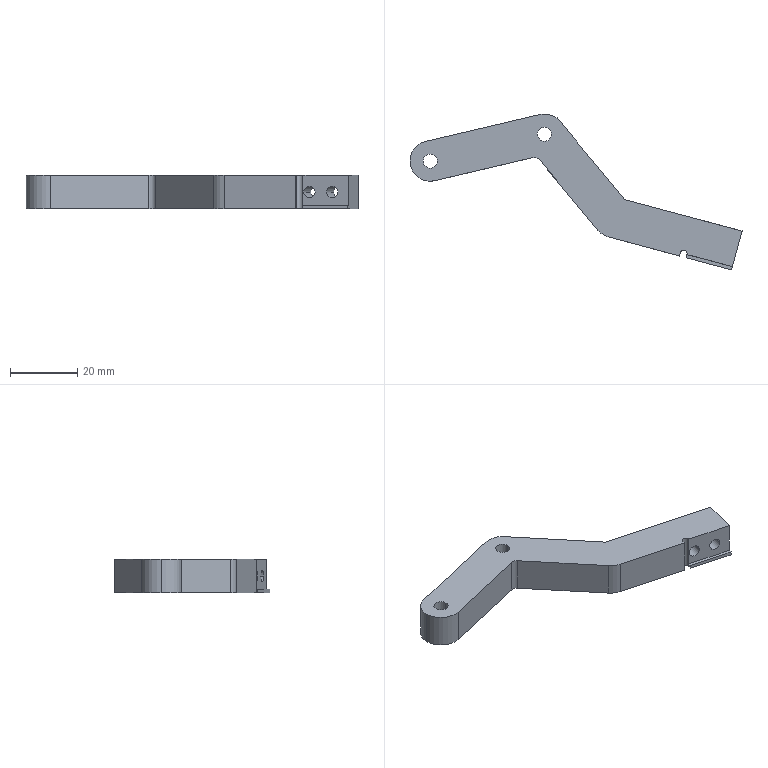Part | STEP file | 02-06 product suction plate b | 1 solid | 39 faces | box 98.778 x 46.377 x 10 mm | volume 12156 mm3 | cylinder 20 | plane 19 | commonest cylinder face diameters 3.5 x4 4.2 x4 12 x4 8 x3 2 x2 10 x2
STEP:
#1=CARTESIAN_POINT('',(35.046,-23.543,5.));
#2=VERTEX_POINT('',#1);
#3=CARTESIAN_POINT('',(38.91,-24.578,9.));
#4=VERTEX_POINT('',#3);
#5=CARTESIAN_POINT('',(38.91,-24.578,5.));
#6=DIRECTION('',(0.2588,0.9659,0.));
#7=DIRECTION('',(-0.9659,0.2588,0.));
#8=AXIS2_PLACEMENT_3D('',#5,#6,#7);
#9=CIRCLE('',#8,4.);
#10=EDGE_CURVE('',#2,#4,#9,.T.);
#11=ORIENTED_EDGE('',*,*,#10,.F.);
#12=CARTESIAN_POINT('',(35.823,-20.645,5.));
#13=VERTEX_POINT('',#12);
#14=CARTESIAN_POINT('',(35.046,-23.543,5.));
#15=DIRECTION('',(0.2588,0.9659,0.));
#16=VECTOR('',#15,1000.);
#17=LINE('',#14,#16);
#18=EDGE_CURVE('',#2,#13,#17,.T.);
#19=ORIENTED_EDGE('',*,*,#18,.T.);
#20=CARTESIAN_POINT('',(39.687,-21.68,9.));
#21=VERTEX_POINT('',#20);
#22=CARTESIAN_POINT('',(39.687,-21.68,5.));
#23=DIRECTION('',(0.2588,0.9659,0.));
#24=DIRECTION('',(-0.9659,0.2588,0.));
#25=AXIS2_PLACEMENT_3D('',#22,#23,#24);
#26=CIRCLE('',#25,4.);
#27=EDGE_CURVE('',#13,#21,#26,.T.);
#28=ORIENTED_EDGE('',*,*,#27,.T.);
#29=CARTESIAN_POINT('',(38.91,-24.578,9.));
#30=DIRECTION('',(0.2588,0.9659,0.));
#31=VECTOR('',#30,1000.);
#32=LINE('',#29,#31);
#33=EDGE_CURVE('',#4,#21,#32,.T.);
#34=ORIENTED_EDGE('',*,*,#33,.F.);
#35=EDGE_LOOP('',(#11,#19,#28,#34));
#36=FACE_OUTER_BOUND('',#35,.T.);
#37=CARTESIAN_POINT('',(38.91,-24.578,5.));
#38=DIRECTION('',(0.2588,0.9659,0.));
#39=DIRECTION('',(-0.9659,0.2588,0.));
#40=AXIS2_PLACEMENT_3D('',#37,#38,#39);
#41=CYLINDRICAL_SURFACE('',#40,4.);
#42=ADVANCED_FACE('',(#36),#41,.F.);
#43=CARTESIAN_POINT('',(34.942,-31.529,0.));
#44=VERTEX_POINT('',#43);
#45=CARTESIAN_POINT('',(32.976,-31.27,0.));
#46=VERTEX_POINT('',#45);
#47=CARTESIAN_POINT('',(33.942,-31.529,0.));
#48=DIRECTION('',(0.,0.,1.));
#49=DIRECTION('',(1.,0.,0.));
#50=AXIS2_PLACEMENT_3D('',#47,#48,#49);
#51=CIRCLE('',#50,1.);
#52=EDGE_CURVE('',#44,#46,#51,.T.);
#53=ORIENTED_EDGE('',*,*,#52,.F.);
#54=CARTESIAN_POINT('',(34.942,-31.529,10.));
#55=VERTEX_POINT('',#54);
#56=CARTESIAN_POINT('',(34.942,-31.529,0.));
#57=DIRECTION('',(0.,0.,1.));
#58=VECTOR('',#57,1000.);
#59=LINE('',#56,#58);
#60=EDGE_CURVE('',#44,#55,#59,.T.);
#61=ORIENTED_EDGE('',*,*,#60,.T.);
#62=CARTESIAN_POINT('',(32.976,-31.27,10.));
#63=VERTEX_POINT('',#62);
#64=CARTESIAN_POINT('',(33.942,-31.529,10.));
#65=DIRECTION('',(0.,0.,1.));
#66=DIRECTION('',(1.,0.,0.));
#67=AXIS2_PLACEMENT_3D('',#64,#65,#66);
#68=CIRCLE('',#67,1.);
#69=EDGE_CURVE('',#55,#63,#68,.T.);
#70=ORIENTED_EDGE('',*,*,#69,.T.);
#71=CARTESIAN_POINT('',(32.976,-31.27,1.));
#72=DIRECTION('',(0.,0.,1.));
#73=VECTOR('',#72,1000.);
#74=LINE('',#71,#73);
#75=EDGE_CURVE('',#46,#63,#74,.T.);
#76=ORIENTED_EDGE('',*,*,#75,.F.);
#77=EDGE_LOOP('',(#53,#61,#70,#76));
#78=FACE_OUTER_BOUND('',#77,.T.);
#79=CARTESIAN_POINT('',(33.942,-31.529,0.));
#80=DIRECTION('',(0.,0.,1.));
#81=DIRECTION('',(1.,0.,0.));
#82=AXIS2_PLACEMENT_3D('',#79,#80,#81);
#83=CYLINDRICAL_SURFACE('',#82,1.);
#84=ADVANCED_FACE('',(#78),#83,.F.);
#85=CARTESIAN_POINT('',(-5.4,4.,10.));
#86=VERTEX_POINT('',#85);
#87=CARTESIAN_POINT('',(-9.6,4.,10.));
#88=VERTEX_POINT('',#87);
#89=CARTESIAN_POINT('',(-7.5,4.,10.));
#90=DIRECTION('',(0.,0.,-1.));
#91=DIRECTION('',(-1.,0.,0.));
#92=AXIS2_PLACEMENT_3D('',#89,#90,#91);
#93=CIRCLE('',#92,2.1);
#94=EDGE_CURVE('',#86,#88,#93,.T.);
#95=ORIENTED_EDGE('',*,*,#94,.F.);
#96=CARTESIAN_POINT('',(-5.4,4.,0.));
#97=VERTEX_POINT('',#96);
#98=CARTESIAN_POINT('',(-5.4,4.,0.));
#99=DIRECTION('',(0.,0.,-1.));
#100=VECTOR('',#99,1000.);
#101=LINE('',#98,#100);
#102=EDGE_CURVE('',#86,#97,#101,.T.);
#103=ORIENTED_EDGE('',*,*,#102,.T.);
#104=CARTESIAN_POINT('',(-9.6,4.,0.));
#105=VERTEX_POINT('',#104);
#106=CARTESIAN_POINT('',(-7.5,4.,0.));
#107=DIRECTION('',(0.,0.,-1.));
#108=DIRECTION('',(-1.,0.,0.));
#109=AXIS2_PLACEMENT_3D('',#106,#107,#108);
#110=CIRCLE('',#109,2.1);
#111=EDGE_CURVE('',#97,#105,#110,.T.);
#112=ORIENTED_EDGE('',*,*,#111,.T.);
#113=CARTESIAN_POINT('',(-9.6,4.,0.));
#114=DIRECTION('',(0.,0.,-1.));
#115=VECTOR('',#114,1000.);
#116=LINE('',#113,#115);
#117=EDGE_CURVE('',#88,#105,#116,.T.);
#118=ORIENTED_EDGE('',*,*,#117,.F.);
#119=EDGE_LOOP('',(#95,#103,#112,#118));
#120=FACE_OUTER_BOUND('',#119,.T.);
#121=CARTESIAN_POINT('',(-7.5,4.,0.));
#122=DIRECTION('',(0.,0.,-1.));
#123=DIRECTION('',(-1.,0.,0.));
#124=AXIS2_PLACEMENT_3D('',#121,#122,#123);
#125=CYLINDRICAL_SURFACE('',#124,2.1);
#126=ADVANCED_FACE('',(#120),#125,.F.);
#127=CARTESIAN_POINT('',(-39.4,-4.,10.));
#128=VERTEX_POINT('',#127);
#129=CARTESIAN_POINT('',(-43.6,-4.,10.));
#130=VERTEX_POINT('',#129);
#131=CARTESIAN_POINT('',(-41.5,-4.,10.));
#132=DIRECTION('',(0.,0.,-1.));
#133=DIRECTION('',(-1.,0.,0.));
#134=AXIS2_PLACEMENT_3D('',#131,#132,#133);
#135=CIRCLE('',#134,2.1);
#136=EDGE_CURVE('',#128,#130,#135,.T.);
#137=ORIENTED_EDGE('',*,*,#136,.F.);
#138=CARTESIAN_POINT('',(-39.4,-4.,1.3));
#139=VERTEX_POINT('',#138);
#140=CARTESIAN_POINT('',(-39.4,-4.,0.));
#141=DIRECTION('',(0.,0.,-1.));
#142=VECTOR('',#141,1000.);
#143=LINE('',#140,#142);
#144=EDGE_CURVE('',#128,#139,#143,.T.);
#145=ORIENTED_EDGE('',*,*,#144,.T.);
#146=CARTESIAN_POINT('',(-43.6,-4.,1.3));
#147=VERTEX_POINT('',#146);
#148=CARTESIAN_POINT('',(-41.5,-4.,1.3));
#149=DIRECTION('',(0.,0.,-1.));
#150=DIRECTION('',(-1.,0.,0.));
#151=AXIS2_PLACEMENT_3D('',#148,#149,#150);
#152=CIRCLE('',#151,2.1);
#153=EDGE_CURVE('',#139,#147,#152,.T.);
#154=ORIENTED_EDGE('',*,*,#153,.T.);
#155=CARTESIAN_POINT('',(-43.6,-4.,0.));
#156=DIRECTION('',(0.,0.,-1.));
#157=VECTOR('',#156,1000.);
#158=LINE('',#155,#157);
#159=EDGE_CURVE('',#130,#147,#158,.T.);
#160=ORIENTED_EDGE('',*,*,#159,.F.);
#161=EDGE_LOOP('',(#137,#145,#154,#160));
#162=FACE_OUTER_BOUND('',#161,.T.);
#163=CARTESIAN_POINT('',(-41.5,-4.,0.));
#164=DIRECTION('',(0.,0.,-1.));
#165=DIRECTION('',(-1.,0.,0.));
#166=AXIS2_PLACEMENT_3D('',#163,#164,#165);
#167=CYLINDRICAL_SURFACE('',#166,2.1);
#168=ADVANCED_FACE('',(#162),#167,.F.);
#169=CARTESIAN_POINT('',(-36.5,-4.,1.3));
#170=VERTEX_POINT('',#169);
#171=CARTESIAN_POINT('',(-46.5,-4.,1.3));
#172=VERTEX_POINT('',#171);
#173=CARTESIAN_POINT('',(-41.5,-4.,1.3));
#174=DIRECTION('',(0.,0.,-1.));
#175=DIRECTION('',(-1.,0.,0.));
#176=AXIS2_PLACEMENT_3D('',#173,#174,#175);
#177=CIRCLE('',#176,5.);
#178=EDGE_CURVE('',#170,#172,#177,.T.);
#179=ORIENTED_EDGE('',*,*,#178,.F.);
#180=CARTESIAN_POINT('',(-36.5,-4.,0.));
#181=VERTEX_POINT('',#180);
#182=CARTESIAN_POINT('',(-36.5,-4.,1.3));
#183=DIRECTION('',(0.,0.,-1.));
#184=VECTOR('',#183,1000.);
#185=LINE('',#182,#184);
#186=EDGE_CURVE('',#170,#181,#185,.T.);
#187=ORIENTED_EDGE('',*,*,#186,.T.);
#188=CARTESIAN_POINT('',(-46.5,-4.,0.));
#189=VERTEX_POINT('',#188);
#190=CARTESIAN_POINT('',(-41.5,-4.,0.));
#191=DIRECTION('',(0.,0.,-1.));
#192=DIRECTION('',(-1.,0.,0.));
#193=AXIS2_PLACEMENT_3D('',#190,#191,#192);
#194=CIRCLE('',#193,5.);
#195=EDGE_CURVE('',#181,#189,#194,.T.);
#196=ORIENTED_EDGE('',*,*,#195,.T.);
#197=CARTESIAN_POINT('',(-46.5,-4.,1.3));
#198=DIRECTION('',(0.,0.,-1.));
#199=VECTOR('',#198,1000.);
#200=LINE('',#197,#199);
#201=EDGE_CURVE('',#172,#189,#200,.T.);
#202=ORIENTED_EDGE('',*,*,#201,.F.);
#203=EDGE_LOOP('',(#179,#187,#196,#202));
#204=FACE_OUTER_BOUND('',#203,.T.);
#205=CARTESIAN_POINT('',(-41.5,-4.,1.3));
#206=DIRECTION('',(0.,0.,-1.));
#207=DIRECTION('',(-1.,0.,0.));
#208=AXIS2_PLACEMENT_3D('',#205,#206,#207);
#209=CYLINDRICAL_SURFACE('',#208,5.);
#210=ADVANCED_FACE('',(#204),#209,.F.);
#211=CARTESIAN_POINT('',(-40.126,-9.841,10.));
#212=VERTEX_POINT('',#211);
#213=CARTESIAN_POINT('',(-47.5,-4.,10.));
#214=VERTEX_POINT('',#213);
#215=CARTESIAN_POINT('',(-41.5,-4.,10.));
#216=DIRECTION('',(0.,0.,-1.));
#217=DIRECTION('',(-1.,0.,0.));
#218=AXIS2_PLACEMENT_3D('',#215,#216,#217);
#219=CIRCLE('',#218,6.);
#220=EDGE_CURVE('',#212,#214,#219,.T.);
#221=ORIENTED_EDGE('',*,*,#220,.T.);
#222=CARTESIAN_POINT('',(-47.5,-4.,0.));
#223=VERTEX_POINT('',#222);
#224=CARTESIAN_POINT('',(-47.5,-4.,10.));
#225=DIRECTION('',(0.,0.,-1.));
#226=VECTOR('',#225,1000.);
#227=LINE('',#224,#226);
#228=EDGE_CURVE('',#214,#223,#227,.T.);
#229=ORIENTED_EDGE('',*,*,#228,.T.);
#230=CARTESIAN_POINT('',(-40.126,-9.841,0.));
#231=VERTEX_POINT('',#230);
#232=CARTESIAN_POINT('',(-41.5,-4.,0.));
#233=DIRECTION('',(0.,0.,-1.));
#234=DIRECTION('',(-1.,0.,0.));
#235=AXIS2_PLACEMENT_3D('',#232,#233,#234);
#236=CIRCLE('',#235,6.);
#237=EDGE_CURVE('',#231,#223,#236,.T.);
#238=ORIENTED_EDGE('',*,*,#237,.F.);
#239=CARTESIAN_POINT('',(-40.126,-9.841,10.));
#240=DIRECTION('',(0.,0.,-1.));
#241=VECTOR('',#240,1000.);
#242=LINE('',#239,#241);
#243=EDGE_CURVE('',#212,#231,#242,.T.);
#244=ORIENTED_EDGE('',*,*,#243,.F.);
#245=EDGE_LOOP('',(#221,#229,#238,#244));
#246=FACE_OUTER_BOUND('',#245,.T.);
#247=CARTESIAN_POINT('',(-41.5,-4.,10.));
#248=DIRECTION('',(0.,0.,-1.));
#249=DIRECTION('',(-1.,0.,0.));
#250=AXIS2_PLACEMENT_3D('',#247,#248,#249);
#251=CYLINDRICAL_SURFACE('',#250,6.);
#252=ADVANCED_FACE('',(#246),#251,.T.);
#253=CARTESIAN_POINT('',(45.291,-34.57,5.));
#254=VERTEX_POINT('',#253);
#255=CARTESIAN_POINT('',(41.911,-33.664,5.));
#256=VERTEX_POINT('',#255);
#257=CARTESIAN_POINT('',(43.601,-34.117,5.));
#258=DIRECTION('',(0.2588,0.9659,0.));
#259=DIRECTION('',(-0.9659,0.2588,0.));
#260=AXIS2_PLACEMENT_3D('',#257,#258,#259);
#261=CIRCLE('',#260,1.75);
#262=EDGE_CURVE('',#254,#256,#261,.T.);
#263=ORIENTED_EDGE('',*,*,#262,.F.);
#264=CARTESIAN_POINT('',(47.362,-26.842,5.));
#265=VERTEX_POINT('',#264);
#266=CARTESIAN_POINT('',(44.256,-38.434,5.));
#267=DIRECTION('',(0.2588,0.9659,0.));
#268=VECTOR('',#267,1000.);
#269=LINE('',#266,#268);
#270=EDGE_CURVE('',#254,#265,#269,.T.);
#271=ORIENTED_EDGE('',*,*,#270,.T.);
#272=CARTESIAN_POINT('',(43.981,-25.937,5.));
#273=VERTEX_POINT('',#272);
#274=CARTESIAN_POINT('',(45.672,-26.39,5.));
#275=DIRECTION('',(-0.2588,-0.9659,0.));
#276=DIRECTION('',(-0.9659,0.2588,0.));
#277=AXIS2_PLACEMENT_3D('',#274,#275,#276);
#278=CIRCLE('',#277,1.75);
#279=EDGE_CURVE('',#273,#265,#278,.T.);
#280=ORIENTED_EDGE('',*,*,#279,.F.);
#281=CARTESIAN_POINT('',(40.875,-37.528,5.));
#282=DIRECTION('',(0.2588,0.9659,0.));
#283=VECTOR('',#282,1000.);
#284=LINE('',#281,#283);
#285=EDGE_CURVE('',#256,#273,#284,.T.);
#286=ORIENTED_EDGE('',*,*,#285,.F.);
#287=EDGE_LOOP('',(#263,#271,#280,#286));
#288=FACE_OUTER_BOUND('',#287,.T.);
#289=CARTESIAN_POINT('',(42.566,-37.981,5.));
#290=DIRECTION('',(0.2588,0.9659,0.));
#291=DIRECTION('',(-0.9659,0.2588,0.));
#292=AXIS2_PLACEMENT_3D('',#289,#290,#291);
#293=CYLINDRICAL_SURFACE('',#292,1.75);
#294=ADVANCED_FACE('',(#288),#293,.F.);
#295=CARTESIAN_POINT('',(38.53,-32.758,5.));
#296=VERTEX_POINT('',#295);
#297=CARTESIAN_POINT('',(35.149,-31.852,5.));
#298=VERTEX_POINT('',#297);
#299=CARTESIAN_POINT('',(36.84,-32.305,5.));
#300=DIRECTION('',(0.2588,0.9659,0.));
#301=DIRECTION('',(-0.9659,0.2588,0.));
#302=AXIS2_PLACEMENT_3D('',#299,#300,#301);
#303=CIRCLE('',#302,1.75);
#304=EDGE_CURVE('',#296,#298,#303,.T.);
#305=ORIENTED_EDGE('',*,*,#304,.F.);
#306=CARTESIAN_POINT('',(40.601,-25.031,5.));
#307=VERTEX_POINT('',#306);
#308=CARTESIAN_POINT('',(37.495,-36.622,5.));
#309=DIRECTION('',(0.2588,0.9659,0.));
#310=VECTOR('',#309,1000.);
#311=LINE('',#308,#310);
#312=EDGE_CURVE('',#296,#307,#311,.T.);
#313=ORIENTED_EDGE('',*,*,#312,.T.);
#314=CARTESIAN_POINT('',(37.22,-24.125,5.));
#315=VERTEX_POINT('',#314);
#316=CARTESIAN_POINT('',(38.91,-24.578,5.));
#317=DIRECTION('',(-0.2588,-0.9659,0.));
#318=DIRECTION('',(-0.9659,0.2588,0.));
#319=AXIS2_PLACEMENT_3D('',#316,#317,#318);
#320=CIRCLE('',#319,1.75);
#321=EDGE_CURVE('',#315,#307,#320,.T.);
#322=ORIENTED_EDGE('',*,*,#321,.F.);
#323=CARTESIAN_POINT('',(34.114,-35.716,5.));
#324=DIRECTION('',(0.2588,0.9659,0.));
#325=VECTOR('',#324,1000.);
#326=LINE('',#323,#325);
#327=EDGE_CURVE('',#298,#315,#326,.T.);
#328=ORIENTED_EDGE('',*,*,#327,.F.);
#329=EDGE_LOOP('',(#305,#313,#322,#328));
#330=FACE_OUTER_BOUND('',#329,.T.);
#331=CARTESIAN_POINT('',(35.804,-36.169,5.));
#332=DIRECTION('',(0.2588,0.9659,0.));
#333=DIRECTION('',(-0.9659,0.2588,0.));
#334=AXIS2_PLACEMENT_3D('',#331,#332,#333);
#335=CYLINDRICAL_SURFACE('',#334,1.75);
#336=ADVANCED_FACE('',(#330),#335,.F.);
#337=ORIENTED_EDGE('',*,*,#312,.F.);
#338=CARTESIAN_POINT('',(36.84,-32.305,5.));
#339=DIRECTION('',(0.2588,0.9659,0.));
#340=DIRECTION('',(-0.9659,0.2588,0.));
#341=AXIS2_PLACEMENT_3D('',#338,#339,#340);
#342=CIRCLE('',#341,1.75);
#343=EDGE_CURVE('',#298,#296,#342,.T.);
#344=ORIENTED_EDGE('',*,*,#343,.F.);
#345=ORIENTED_EDGE('',*,*,#327,.T.);
#346=CARTESIAN_POINT('',(38.91,-24.578,5.));
#347=DIRECTION('',(-0.2588,-0.9659,0.));
#348=DIRECTION('',(-0.9659,0.2588,0.));
#349=AXIS2_PLACEMENT_3D('',#346,#347,#348);
#350=CIRCLE('',#349,1.75);
#351=EDGE_CURVE('',#307,#315,#350,.T.);
#352=ORIENTED_EDGE('',*,*,#351,.F.);
#353=EDGE_LOOP('',(#337,#344,#345,#352));
#354=FACE_OUTER_BOUND('',#353,.T.);
#355=CARTESIAN_POINT('',(35.804,-36.169,5.));
#356=DIRECTION('',(0.2588,0.9659,0.));
#357=DIRECTION('',(-0.9659,0.2588,0.));
#358=AXIS2_PLACEMENT_3D('',#355,#356,#357);
#359=CYLINDRICAL_SURFACE('',#358,1.75);
#360=ADVANCED_FACE('',(#354),#359,.F.);
#361=ORIENTED_EDGE('',*,*,#270,.F.);
#362=CARTESIAN_POINT('',(43.601,-34.117,5.));
#363=DIRECTION('',(0.2588,0.9659,0.));
#364=DIRECTION('',(-0.9659,0.2588,0.));
#365=AXIS2_PLACEMENT_3D('',#362,#363,#364);
#366=CIRCLE('',#365,1.75);
#367=EDGE_CURVE('',#256,#254,#366,.T.);
#368=ORIENTED_EDGE('',*,*,#367,.F.);
#369=ORIENTED_EDGE('',*,*,#285,.T.);
#370=CARTESIAN_POINT('',(45.672,-26.39,5.));
#371=DIRECTION('',(-0.2588,-0.9659,0.));
#372=DIRECTION('',(-0.9659,0.2588,0.));
#373=AXIS2_PLACEMENT_3D('',#370,#371,#372);
#374=CIRCLE('',#373,1.75);
#375=EDGE_CURVE('',#265,#273,#374,.T.);
#376=ORIENTED_EDGE('',*,*,#375,.F.);
#377=EDGE_LOOP('',(#361,#368,#369,#376));
#378=FACE_OUTER_BOUND('',#377,.T.);
#379=CARTESIAN_POINT('',(42.566,-37.981,5.));
#380=DIRECTION('',(0.2588,0.9659,0.));
#381=DIRECTION('',(-0.9659,0.2588,0.));
#382=AXIS2_PLACEMENT_3D('',#379,#380,#381);
#383=CYLINDRICAL_SURFACE('',#382,1.75);
#384=ADVANCED_FACE('',(#378),#383,.F.);
#385=CARTESIAN_POINT('',(34.649,-32.754,0.));
#386=VERTEX_POINT('',#385);
#387=CARTESIAN_POINT('',(34.649,-32.754,1.));
#388=VERTEX_POINT('',#387);
#389=CARTESIAN_POINT('',(34.649,-32.754,10.));
#390=DIRECTION('',(0.,0.,1.));
#391=VECTOR('',#390,1000.);
#392=LINE('',#389,#391);
#393=EDGE_CURVE('',#386,#388,#392,.T.);
#394=ORIENTED_EDGE('',*,*,#393,.F.);
#395=CARTESIAN_POINT('',(48.172,-36.377,0.));
#396=VERTEX_POINT('',#395);
#397=CARTESIAN_POINT('',(48.172,-36.377,0.));
#398=DIRECTION('',(-0.9659,0.2588,0.));
#399=VECTOR('',#398,1000.);
#400=LINE('',#397,#399);
#401=EDGE_CURVE('',#396,#386,#400,.T.);
#402=ORIENTED_EDGE('',*,*,#401,.F.);
#403=CARTESIAN_POINT('',(48.172,-36.377,1.));
#404=VERTEX_POINT('',#403);
#405=CARTESIAN_POINT('',(48.172,-36.377,10.));
#406=DIRECTION('',(0.,0.,-1.));
#407=VECTOR('',#406,1000.);
#408=LINE('',#405,#407);
#409=EDGE_CURVE('',#404,#396,#408,.T.);
#410=ORIENTED_EDGE('',*,*,#409,.F.);
#411=CARTESIAN_POINT('',(32.717,-32.236,1.));
#412=DIRECTION('',(0.9659,-0.2588,0.));
#413=VECTOR('',#412,1000.);
#414=LINE('',#411,#413);
#415=EDGE_CURVE('',#388,#404,#414,.T.);
#416=ORIENTED_EDGE('',*,*,#415,.F.);
#417=EDGE_LOOP('',(#394,#402,#410,#416));
#418=FACE_OUTER_BOUND('',#417,.T.);
#419=CARTESIAN_POINT('',(48.172,-36.377,10.));
#420=DIRECTION('',(-0.2588,-0.9659,0.));
#421=DIRECTION('',(0.9659,-0.2588,0.));
#422=AXIS2_PLACEMENT_3D('',#419,#420,#421);
#423=PLANE('',#422);
#424=ADVANCED_FACE('',(#418),#423,.T.);
#425=CARTESIAN_POINT('',(32.717,-32.236,0.));
#426=VERTEX_POINT('',#425);
#427=CARTESIAN_POINT('',(11.467,-26.542,0.));
#428=VERTEX_POINT('',#427);
#429=CARTESIAN_POINT('',(48.172,-36.377,0.));
#430=DIRECTION('',(-0.9659,0.2588,0.));
#431=VECTOR('',#430,1000.);
#432=LINE('',#429,#431);
#433=EDGE_CURVE('',#426,#428,#432,.T.);
#434=ORIENTED_EDGE('',*,*,#433,.F.);
#435=CARTESIAN_POINT('',(32.717,-32.236,10.));
#436=VERTEX_POINT('',#435);
#437=CARTESIAN_POINT('',(32.717,-32.236,1.));
#438=DIRECTION('',(0.,0.,1.));
#439=VECTOR('',#438,1000.);
#440=LINE('',#437,#439);
#441=EDGE_CURVE('',#426,#436,#440,.T.);
#442=ORIENTED_EDGE('',*,*,#441,.T.);
#443=CARTESIAN_POINT('',(11.467,-26.542,10.));
#444=VERTEX_POINT('',#443);
#445=CARTESIAN_POINT('',(48.172,-36.377,10.));
#446=DIRECTION('',(-0.9659,0.2588,0.));
#447=VECTOR('',#446,1000.);
#448=LINE('',#445,#447);
#449=EDGE_CURVE('',#436,#444,#448,.T.);
#450=ORIENTED_EDGE('',*,*,#449,.T.);
#451=CARTESIAN_POINT('',(11.467,-26.542,10.));
#452=DIRECTION('',(0.,0.,-1.));
#453=VECTOR('',#452,1000.);
#454=LINE('',#451,#453);
#455=EDGE_CURVE('',#444,#428,#454,.T.);
#456=ORIENTED_EDGE('',*,*,#455,.T.);
#457=EDGE_LOOP('',(#434,#442,#450,#456));
#458=FACE_OUTER_BOUND('',#457,.T.);
#459=CARTESIAN_POINT('',(48.172,-36.377,10.));
#460=DIRECTION('',(-0.2588,-0.9659,0.));
#461=DIRECTION('',(0.9659,-0.2588,0.));
#462=AXIS2_PLACEMENT_3D('',#459,#460,#461);
#463=PLANE('',#462);
#464=ADVANCED_FACE('',(#458),#463,.T.);
#465=CARTESIAN_POINT('',(48.431,-35.411,1.));
#466=VERTEX_POINT('',#465);
#467=CARTESIAN_POINT('',(48.431,-35.411,10.));
#468=VERTEX_POINT('',#467);
#469=CARTESIAN_POINT('',(48.431,-35.411,1.));
#470=DIRECTION('',(0.,0.,1.));
#471=VECTOR('',#470,1000.);
#472=LINE('',#469,#471);
#473=EDGE_CURVE('',#466,#468,#472,.T.);
#474=ORIENTED_EDGE('',*,*,#473,.F.);
#475=CARTESIAN_POINT('',(48.172,-36.377,1.));
#476=DIRECTION('',(0.2588,0.9659,0.));
#477=VECTOR('',#476,1000.);
#478=LINE('',#475,#477);
#479=EDGE_CURVE('',#404,#466,#478,.T.);
#480=ORIENTED_EDGE('',*,*,#479,.F.);
#481=ORIENTED_EDGE('',*,*,#409,.T.);
#482=CARTESIAN_POINT('',(51.278,-24.786,0.));
#483=VERTEX_POINT('',#482);
#484=CARTESIAN_POINT('',(53.31,-17.202,0.));
#485=DIRECTION('',(-0.2588,-0.9659,0.));
#486=VECTOR('',#485,1000.);
#487=LINE('',#484,#486);
#488=EDGE_CURVE('',#483,#396,#487,.T.);
#489=ORIENTED_EDGE('',*,*,#488,.F.);
#490=CARTESIAN_POINT('',(51.278,-24.786,10.));
#491=VERTEX_POINT('',#490);
#492=CARTESIAN_POINT('',(51.278,-24.786,0.));
#493=DIRECTION('',(0.,0.,1.));
#494=VECTOR('',#493,1000.);
#495=LINE('',#492,#494);
#496=EDGE_CURVE('',#483,#491,#495,.T.);
#497=ORIENTED_EDGE('',*,*,#496,.T.);
#498=CARTESIAN_POINT('',(53.31,-17.202,10.));
#499=DIRECTION('',(-0.2588,-0.9659,0.));
#500=VECTOR('',#499,1000.);
#501=LINE('',#498,#500);
#502=EDGE_CURVE('',#491,#468,#501,.T.);
#503=ORIENTED_EDGE('',*,*,#502,.T.);
#504=EDGE_LOOP('',(#474,#480,#481,#489,#497,#503));
#505=FACE_OUTER_BOUND('',#504,.T.);
#506=CARTESIAN_POINT('',(53.31,-17.202,10.));
#507=DIRECTION('',(0.9659,-0.2588,0.));
#508=DIRECTION('',(0.2588,0.9659,0.));
#509=AXIS2_PLACEMENT_3D('',#506,#507,#508);
#510=PLANE('',#509);
#511=ADVANCED_FACE('',(#505),#510,.T.);
#512=CARTESIAN_POINT('',(-5.005,9.457,0.));
#513=VERTEX_POINT('',#512);
#514=CARTESIAN_POINT('',(-3.757,8.886,0.));
#515=VERTEX_POINT('',#514);
#516=CARTESIAN_POINT('',(-6.874,10.311,0.));
#517=DIRECTION('',(0.9095,-0.4158,0.));
#518=VECTOR('',#517,1000.);
#519=LINE('',#516,#518);
#520=EDGE_CURVE('',#513,#515,#519,.T.);
#521=ORIENTED_EDGE('',*,*,#520,.F.);
#522=CARTESIAN_POINT('',(-5.005,9.457,10.));
#523=VERTEX_POINT('',#522);
#524=CARTESIAN_POINT('',(-5.005,9.457,10.));
#525=DIRECTION('',(0.,0.,1.));
#526=VECTOR('',#525,1000.);
#527=LINE('',#524,#526);
#528=EDGE_CURVE('',#513,#523,#527,.T.);
#529=ORIENTED_EDGE('',*,*,#528,.T.);
#530=CARTESIAN_POINT('',(-3.757,8.886,10.));
#531=VERTEX_POINT('',#530);
#532=CARTESIAN_POINT('',(-6.874,10.311,10.));
#533=DIRECTION('',(0.9095,-0.4158,0.));
#534=VECTOR('',#533,1000.);
#535=LINE('',#532,#534);
#536=EDGE_CURVE('',#523,#531,#535,.T.);
#537=ORIENTED_EDGE('',*,*,#536,.T.);
#538=CARTESIAN_POINT('',(-3.757,8.886,0.));
#539=DIRECTION('',(0.,0.,1.));
#540=VECTOR('',#539,1000.);
#541=LINE('',#538,#540);
#542=EDGE_CURVE('',#515,#531,#541,.T.);
#543=ORIENTED_EDGE('',*,*,#542,.F.);
#544=EDGE_LOOP('',(#521,#529,#537,#543));
#545=FACE_OUTER_BOUND('',#544,.T.);
#546=CARTESIAN_POINT('',(-6.874,10.311,10.));
#547=DIRECTION('',(0.4158,0.9095,0.));
#548=DIRECTION('',(-0.9095,0.4158,0.));
#549=AXIS2_PLACEMENT_3D('',#546,#547,#548);
#550=PLANE('',#549);
#551=ADVANCED_FACE('',(#545),#550,.T.);
#552=CARTESIAN_POINT('',(-42.874,1.841,10.));
#553=VERTEX_POINT('',#552);
#554=CARTESIAN_POINT('',(-8.874,9.841,10.));
#555=VERTEX_POINT('',#554);
#556=CARTESIAN_POINT('',(-42.874,1.841,10.));
#557=DIRECTION('',(0.9734,0.229,0.));
#558=VECTOR('',#557,1000.);
#559=LINE('',#556,#558);
#560=EDGE_CURVE('',#553,#555,#559,.T.);
#561=ORIENTED_EDGE('',*,*,#560,.T.);
#562=CARTESIAN_POINT('',(-8.874,9.841,0.));
#563=VERTEX_POINT('',#562);
#564=CARTESIAN_POINT('',(-8.874,9.841,10.));
#565=DIRECTION('',(0.,0.,-1.));
#566=VECTOR('',#565,1000.);
#567=LINE('',#564,#566);
#568=EDGE_CURVE('',#555,#563,#567,.T.);
#569=ORIENTED_EDGE('',*,*,#568,.T.);
#570=CARTESIAN_POINT('',(-42.874,1.841,0.));
#571=VERTEX_POINT('',#570);
#572=CARTESIAN_POINT('',(-42.874,1.841,0.));
#573=DIRECTION('',(0.9734,0.229,0.));
#574=VECTOR('',#573,1000.);
#575=LINE('',#572,#574);
#576=EDGE_CURVE('',#571,#563,#575,.T.);
#577=ORIENTED_EDGE('',*,*,#576,.F.);
#578=CARTESIAN_POINT('',(-42.874,1.841,10.));
#579=DIRECTION('',(0.,0.,-1.));
#580=VECTOR('',#579,1000.);
#581=LINE('',#578,#580);
#582=EDGE_CURVE('',#553,#571,#581,.T.);
#583=ORIENTED_EDGE('',*,*,#582,.F.);
#584=EDGE_LOOP('',(#561,#569,#577,#583));
#585=FACE_OUTER_BOUND('',#584,.T.);
#586=CARTESIAN_POINT('',(-42.874,1.841,10.));
#587=DIRECTION('',(-0.229,0.9734,0.));
#588=DIRECTION('',(-0.9734,-0.229,0.));
#589=AXIS2_PLACEMENT_3D('',#586,#587,#588);
#590=PLANE('',#589);
#591=ADVANCED_FACE('',(#585),#590,.T.);
#592=ORIENTED_EDGE('',*,*,#228,.F.);
#593=CARTESIAN_POINT('',(-41.5,-4.,10.));
#594=DIRECTION('',(0.,0.,-1.));
#595=DIRECTION('',(-1.,0.,0.));
#596=AXIS2_PLACEMENT_3D('',#593,#594,#595);
#597=CIRCLE('',#596,6.);
#598=EDGE_CURVE('',#214,#553,#597,.T.);
#599=ORIENTED_EDGE('',*,*,#598,.T.);
#600=ORIENTED_EDGE('',*,*,#582,.T.);
#601=CARTESIAN_POINT('',(-41.5,-4.,0.));
#602=DIRECTION('',(0.,0.,-1.));
#603=DIRECTION('',(-1.,0.,0.));
#604=AXIS2_PLACEMENT_3D('',#601,#602,#603);
#605=CIRCLE('',#604,6.);
#606=EDGE_CURVE('',#223,#571,#605,.T.);
#607=ORIENTED_EDGE('',*,*,#606,.F.);
#608=EDGE_LOOP('',(#592,#599,#600,#607));
#609=FACE_OUTER_BOUND('',#608,.T.);
#610=CARTESIAN_POINT('',(-41.5,-4.,10.));
#611=DIRECTION('',(0.,0.,-1.));
#612=DIRECTION('',(-1.,0.,0.));
#613=AXIS2_PLACEMENT_3D('',#610,#611,#612);
#614=CYLINDRICAL_SURFACE('',#613,6.);
#615=ADVANCED_FACE('',(#609),#614,.T.);
#616=CARTESIAN_POINT('',(-10.952,-2.976,0.));
#617=VERTEX_POINT('',#616);
#618=CARTESIAN_POINT('',(-9.745,-2.692,0.));
#619=DIRECTION('',(-0.9734,-0.229,0.));
#620=VECTOR('',#619,1000.);
#621=LINE('',#618,#620);
#622=EDGE_CURVE('',#617,#231,#621,.T.);
#623=ORIENTED_EDGE('',*,*,#622,.F.);
#624=CARTESIAN_POINT('',(-10.952,-2.976,10.));
#625=VERTEX_POINT('',#624);
#626=CARTESIAN_POINT('',(-10.952,-2.976,10.));
#627=DIRECTION('',(0.,0.,1.));
#628=VECTOR('',#627,1000.);
#629=LINE('',#626,#628);
#630=EDGE_CURVE('',#617,#625,#629,.T.);
#631=ORIENTED_EDGE('',*,*,#630,.T.);
#632=CARTESIAN_POINT('',(-9.745,-2.692,10.));
#633=DIRECTION('',(-0.9734,-0.229,0.));
#634=VECTOR('',#633,1000.);
#635=LINE('',#632,#634);
#636=EDGE_CURVE('',#625,#212,#635,.T.);
#637=ORIENTED_EDGE('',*,*,#636,.T.);
#638=ORIENTED_EDGE('',*,*,#243,.T.);
#639=EDGE_LOOP('',(#623,#631,#637,#638));
#640=FACE_OUTER_BOUND('',#639,.T.);
#641=CARTESIAN_POINT('',(-9.745,-2.692,10.));
#642=DIRECTION('',(0.229,-0.9734,0.));
#643=DIRECTION('',(0.9734,0.229,0.));
#644=AXIS2_PLACEMENT_3D('',#641,#642,#643);
#645=PLANE('',#644);
#646=ADVANCED_FACE('',(#640),#645,.T.);
#647=CARTESIAN_POINT('',(8.401,-24.576,0.));
#648=VERTEX_POINT('',#647);
#649=CARTESIAN_POINT('',(-8.954,-3.646,0.));
#650=VERTEX_POINT('',#649);
#651=CARTESIAN_POINT('',(9.621,-26.047,0.));
#652=DIRECTION('',(-0.6383,0.7698,0.));
#653=VECTOR('',#652,1000.);
#654=LINE('',#651,#653);
#655=EDGE_CURVE('',#648,#650,#654,.T.);
#656=ORIENTED_EDGE('',*,*,#655,.F.);
#657=CARTESIAN_POINT('',(8.401,-24.576,10.));
#658=VERTEX_POINT('',#657);
#659=CARTESIAN_POINT('',(8.401,-24.576,10.));
#660=DIRECTION('',(0.,0.,1.));
#661=VECTOR('',#660,1000.);
#662=LINE('',#659,#661);
#663=EDGE_CURVE('',#648,#658,#662,.T.);
#664=ORIENTED_EDGE('',*,*,#663,.T.);
#665=CARTESIAN_POINT('',(-8.954,-3.646,10.));
#666=VERTEX_POINT('',#665);
#667=CARTESIAN_POINT('',(9.621,-26.047,10.));
#668=DIRECTION('',(-0.6383,0.7698,0.));
#669=VECTOR('',#668,1000.);
#670=LINE('',#667,#669);
#671=EDGE_CURVE('',#658,#666,#670,.T.);
#672=ORIENTED_EDGE('',*,*,#671,.T.);
#673=CARTESIAN_POINT('',(-8.954,-3.646,0.));
#674=DIRECTION('',(0.,0.,-1.));
#675=VECTOR('',#674,1000.);
#676=LINE('',#673,#675);
#677=EDGE_CURVE('',#666,#650,#676,.T.);
#678=ORIENTED_EDGE('',*,*,#677,.T.);
#679=EDGE_LOOP('',(#656,#664,#672,#678));
#680=FACE_OUTER_BOUND('',#679,.T.);
#681=CARTESIAN_POINT('',(9.621,-26.047,10.));
#682=DIRECTION('',(-0.7698,-0.6383,0.));
#683=DIRECTION('',(0.6383,-0.7698,0.));
#684=AXIS2_PLACEMENT_3D('',#681,#682,#683);
#685=PLANE('',#684);
#686=ADVANCED_FACE('',(#680),#685,.T.);
#687=CARTESIAN_POINT('',(-7.5,4.,10.));
#688=DIRECTION('',(0.,0.,-1.));
#689=DIRECTION('',(-1.,0.,0.));
#690=AXIS2_PLACEMENT_3D('',#687,#688,#689);
#691=CIRCLE('',#690,2.1);
#692=EDGE_CURVE('',#88,#86,#691,.T.);
#693=ORIENTED_EDGE('',*,*,#692,.T.);
#694=ORIENTED_EDGE('',*,*,#94,.T.);
#695=EDGE_LOOP('',(#693,#694));
#696=FACE_BOUND('',#695,.T.);
#697=CARTESIAN_POINT('',(-41.5,-4.,10.));
#698=DIRECTION('',(0.,0.,-1.));
#699=DIRECTION('',(-1.,0.,0.));
#700=AXIS2_PLACEMENT_3D('',#697,#698,#699);
#701=CIRCLE('',#700,2.1);
#702=EDGE_CURVE('',#130,#128,#701,.T.);
#703=ORIENTED_EDGE('',*,*,#702,.T.);
#704=ORIENTED_EDGE('',*,*,#136,.T.);
#705=EDGE_LOOP('',(#703,#704));
#706=FACE_BOUND('',#705,.T.);
#707=CARTESIAN_POINT('',(32.717,-32.236,10.));
#708=DIRECTION('',(-0.2588,-0.9659,0.));
#709=VECTOR('',#708,1000.);
#710=LINE('',#707,#709);
#711=EDGE_CURVE('',#63,#436,#710,.T.);
#712=ORIENTED_EDGE('',*,*,#711,.F.);
#713=ORIENTED_EDGE('',*,*,#69,.F.);
#714=CARTESIAN_POINT('',(34.908,-31.788,10.));
#715=VERTEX_POINT('',#714);
#716=CARTESIAN_POINT('',(33.942,-31.529,10.));
#717=DIRECTION('',(0.,0.,1.));
#718=DIRECTION('',(1.,0.,0.));
#719=AXIS2_PLACEMENT_3D('',#716,#717,#718);
#720=CIRCLE('',#719,1.);
#721=EDGE_CURVE('',#715,#55,#720,.T.);
#722=ORIENTED_EDGE('',*,*,#721,.F.);
#723=CARTESIAN_POINT('',(48.431,-35.411,10.));
#724=DIRECTION('',(-0.9659,0.2588,0.));
#725=VECTOR('',#724,1000.);
#726=LINE('',#723,#725);
#727=EDGE_CURVE('',#468,#715,#726,.T.);
#728=ORIENTED_EDGE('',*,*,#727,.F.);
#729=ORIENTED_EDGE('',*,*,#502,.F.);
#730=CARTESIAN_POINT('',(16.419,-15.445,10.));
#731=VERTEX_POINT('',#730);
#732=CARTESIAN_POINT('',(16.419,-15.445,10.));
#733=DIRECTION('',(0.9659,-0.2588,0.));
#734=VECTOR('',#733,1000.);
#735=LINE('',#732,#734);
#736=EDGE_CURVE('',#731,#491,#735,.T.);
#737=ORIENTED_EDGE('',*,*,#736,.F.);
#738=CARTESIAN_POINT('',(-3.757,8.886,10.));
#739=DIRECTION('',(0.6383,-0.7698,0.));
#740=VECTOR('',#739,1000.);
#741=LINE('',#738,#740);
#742=EDGE_CURVE('',#531,#731,#741,.T.);
#743=ORIENTED_EDGE('',*,*,#742,.F.);
#744=ORIENTED_EDGE('',*,*,#536,.F.);
#745=CARTESIAN_POINT('',(-7.5,4.,10.));
#746=DIRECTION('',(0.,0.,1.));
#747=DIRECTION('',(-1.,0.,0.));
#748=AXIS2_PLACEMENT_3D('',#745,#746,#747);
#749=CIRCLE('',#748,6.);
#750=EDGE_CURVE('',#523,#555,#749,.T.);
#751=ORIENTED_EDGE('',*,*,#750,.T.);
#752=ORIENTED_EDGE('',*,*,#560,.F.);
#753=ORIENTED_EDGE('',*,*,#598,.F.);
#754=ORIENTED_EDGE('',*,*,#220,.F.);
#755=ORIENTED_EDGE('',*,*,#636,.F.);
#756=CARTESIAN_POINT('',(-10.494,-4.923,10.));
#757=DIRECTION('',(0.,0.,-1.));
#758=DIRECTION('',(-1.,0.,0.));
#759=AXIS2_PLACEMENT_3D('',#756,#757,#758);
#760=CIRCLE('',#759,2.);
#761=EDGE_CURVE('',#625,#666,#760,.T.);
#762=ORIENTED_EDGE('',*,*,#761,.T.);
#763=ORIENTED_EDGE('',*,*,#671,.F.);
#764=CARTESIAN_POINT('',(13.02,-20.746,10.));
#765=DIRECTION('',(0.,0.,1.));
#766=DIRECTION('',(-1.,0.,0.));
#767=AXIS2_PLACEMENT_3D('',#764,#765,#766);
#768=CIRCLE('',#767,6.);
#769=EDGE_CURVE('',#658,#444,#768,.T.);
#770=ORIENTED_EDGE('',*,*,#769,.T.);
#771=ORIENTED_EDGE('',*,*,#449,.F.);
#772=EDGE_LOOP('',(#712,#713,#722,#728,#729,#737,#743,#744,#751,#752,#753,#754,#755,#762,#763,#770,#771));
#773=FACE_OUTER_BOUND('',#772,.T.);
#774=CARTESIAN_POINT('',(-41.5,-4.,10.));
#775=DIRECTION('',(0.,0.,-1.));
#776=DIRECTION('',(-1.,0.,0.));
#777=AXIS2_PLACEMENT_3D('',#774,#775,#776);
#778=PLANE('',#777);
#779=ADVANCED_FACE('',(#696,#706,#773),#778,.F.);
#780=CARTESIAN_POINT('',(34.908,-31.788,0.));
#781=VERTEX_POINT('',#780);
#782=CARTESIAN_POINT('',(34.908,-31.788,0.));
#783=DIRECTION('',(0.2588,0.9659,0.));
#784=VECTOR('',#783,1000.);
#785=LINE('',#782,#784);
#786=EDGE_CURVE('',#386,#781,#785,.T.);
#787=ORIENTED_EDGE('',*,*,#786,.T.);
#788=CARTESIAN_POINT('',(33.942,-31.529,0.));
#789=DIRECTION('',(0.,0.,1.));
#790=DIRECTION('',(1.,0.,0.));
#791=AXIS2_PLACEMENT_3D('',#788,#789,#790);
#792=CIRCLE('',#791,1.);
#793=EDGE_CURVE('',#781,#44,#792,.T.);
#794=ORIENTED_EDGE('',*,*,#793,.T.);
#795=ORIENTED_EDGE('',*,*,#52,.T.);
#796=CARTESIAN_POINT('',(32.976,-31.27,0.));
#797=DIRECTION('',(-0.2588,-0.9659,0.));
#798=VECTOR('',#797,1000.);
#799=LINE('',#796,#798);
#800=EDGE_CURVE('',#46,#426,#799,.T.);
#801=ORIENTED_EDGE('',*,*,#800,.T.);
#802=ORIENTED_EDGE('',*,*,#433,.T.);
#803=CARTESIAN_POINT('',(13.02,-20.746,0.));
#804=DIRECTION('',(0.,0.,-1.));
#805=DIRECTION('',(-1.,0.,0.));
#806=AXIS2_PLACEMENT_3D('',#803,#804,#805);
#807=CIRCLE('',#806,6.);
#808=EDGE_CURVE('',#428,#648,#807,.T.);
#809=ORIENTED_EDGE('',*,*,#808,.T.);
#810=ORIENTED_EDGE('',*,*,#655,.T.);
#811=CARTESIAN_POINT('',(-10.494,-4.923,0.));
#812=DIRECTION('',(0.,0.,1.));
#813=DIRECTION('',(-1.,0.,0.));
#814=AXIS2_PLACEMENT_3D('',#811,#812,#813);
#815=CIRCLE('',#814,2.);
#816=EDGE_CURVE('',#650,#617,#815,.T.);
#817=ORIENTED_EDGE('',*,*,#816,.T.);
#818=ORIENTED_EDGE('',*,*,#622,.T.);
#819=ORIENTED_EDGE('',*,*,#237,.T.);
#820=ORIENTED_EDGE('',*,*,#606,.T.);
#821=ORIENTED_EDGE('',*,*,#576,.T.);
#822=CARTESIAN_POINT('',(-7.5,4.,0.));
#823=DIRECTION('',(0.,0.,-1.));
#824=DIRECTION('',(-1.,0.,0.));
#825=AXIS2_PLACEMENT_3D('',#822,#823,#824);
#826=CIRCLE('',#825,6.);
#827=EDGE_CURVE('',#563,#513,#826,.T.);
#828=ORIENTED_EDGE('',*,*,#827,.T.);
#829=ORIENTED_EDGE('',*,*,#520,.T.);
#830=CARTESIAN_POINT('',(16.419,-15.445,0.));
#831=VERTEX_POINT('',#830);
#832=CARTESIAN_POINT('',(-3.757,8.886,0.));
#833=DIRECTION('',(0.6383,-0.7698,0.));
#834=VECTOR('',#833,1000.);
#835=LINE('',#832,#834);
#836=EDGE_CURVE('',#515,#831,#835,.T.);
#837=ORIENTED_EDGE('',*,*,#836,.T.);
#838=CARTESIAN_POINT('',(16.419,-15.445,0.));
#839=DIRECTION('',(0.9659,-0.2588,0.));
#840=VECTOR('',#839,1000.);
#841=LINE('',#838,#840);
#842=EDGE_CURVE('',#831,#483,#841,.T.);
#843=ORIENTED_EDGE('',*,*,#842,.T.);
#844=ORIENTED_EDGE('',*,*,#488,.T.);
#845=ORIENTED_EDGE('',*,*,#401,.T.);
#846=EDGE_LOOP('',(#787,#794,#795,#801,#802,#809,#810,#817,#818,#819,#820,#821,#828,#829,#837,#843,#844,#845));
#847=FACE_OUTER_BOUND('',#846,.T.);
#848=CARTESIAN_POINT('',(-7.5,4.,0.));
#849=DIRECTION('',(0.,0.,-1.));
#850=DIRECTION('',(-1.,0.,0.));
#851=AXIS2_PLACEMENT_3D('',#848,#849,#850);
#852=CIRCLE('',#851,2.1);
#853=EDGE_CURVE('',#105,#97,#852,.T.);
#854=ORIENTED_EDGE('',*,*,#853,.F.);
#855=ORIENTED_EDGE('',*,*,#111,.F.);
#856=EDGE_LOOP('',(#854,#855));
#857=FACE_BOUND('',#856,.T.);
#858=CARTESIAN_POINT('',(-41.5,-4.,0.));
#859=DIRECTION('',(0.,0.,-1.));
#860=DIRECTION('',(-1.,0.,0.));
#861=AXIS2_PLACEMENT_3D('',#858,#859,#860);
#862=CIRCLE('',#861,5.);
#863=EDGE_CURVE('',#189,#181,#862,.T.);
#864=ORIENTED_EDGE('',*,*,#863,.F.);
#865=ORIENTED_EDGE('',*,*,#195,.F.);
#866=EDGE_LOOP('',(#864,#865));
#867=FACE_BOUND('',#866,.T.);
#868=CARTESIAN_POINT('',(-41.5,-4.,0.));
#869=DIRECTION('',(0.,0.,-1.));
#870=DIRECTION('',(-1.,0.,0.));
#871=AXIS2_PLACEMENT_3D('',#868,#869,#870);
#872=PLANE('',#871);
#873=ADVANCED_FACE('',(#847,#857,#867),#872,.T.);
#874=ORIENTED_EDGE('',*,*,#742,.T.);
#875=CARTESIAN_POINT('',(16.419,-15.445,0.));
#876=DIRECTION('',(0.,0.,1.));
#877=VECTOR('',#876,1000.);
#878=LINE('',#875,#877);
#879=EDGE_CURVE('',#831,#731,#878,.T.);
#880=ORIENTED_EDGE('',*,*,#879,.F.);
#881=ORIENTED_EDGE('',*,*,#836,.F.);
#882=ORIENTED_EDGE('',*,*,#542,.T.);
#883=EDGE_LOOP('',(#874,#880,#881,#882));
#884=FACE_OUTER_BOUND('',#883,.T.);
#885=CARTESIAN_POINT('',(-3.757,8.886,0.));
#886=DIRECTION('',(-0.7698,-0.6383,0.));
#887=DIRECTION('',(0.6383,-0.7698,0.));
#888=AXIS2_PLACEMENT_3D('',#885,#886,#887);
#889=PLANE('',#888);
#890=ADVANCED_FACE('',(#884),#889,.F.);
#891=CARTESIAN_POINT('',(46.448,-23.492,9.));
#892=VERTEX_POINT('',#891);
#893=CARTESIAN_POINT('',(39.687,-21.68,9.));
#894=DIRECTION('',(0.9659,-0.2588,0.));
#895=VECTOR('',#894,1000.);
#896=LINE('',#893,#895);
#897=EDGE_CURVE('',#21,#892,#896,.T.);
#898=ORIENTED_EDGE('',*,*,#897,.F.);
#899=ORIENTED_EDGE('',*,*,#27,.F.);
#900=CARTESIAN_POINT('',(39.687,-21.68,1.));
#901=VERTEX_POINT('',#900);
#902=CARTESIAN_POINT('',(39.687,-21.68,5.));
#903=DIRECTION('',(0.2588,0.9659,0.));
#904=DIRECTION('',(-0.9659,0.2588,0.));
#905=AXIS2_PLACEMENT_3D('',#902,#903,#904);
#906=CIRCLE('',#905,4.);
#907=EDGE_CURVE('',#901,#13,#906,.T.);
#908=ORIENTED_EDGE('',*,*,#907,.F.);
#909=CARTESIAN_POINT('',(46.448,-23.492,1.));
#910=VERTEX_POINT('',#909);
#911=CARTESIAN_POINT('',(39.687,-21.68,1.));
#912=DIRECTION('',(-0.9659,0.2588,0.));
#913=VECTOR('',#912,1000.);
#914=LINE('',#911,#913);
#915=EDGE_CURVE('',#910,#901,#914,.T.);
#916=ORIENTED_EDGE('',*,*,#915,.F.);
#917=CARTESIAN_POINT('',(46.448,-23.492,5.));
#918=DIRECTION('',(0.2588,0.9659,0.));
#919=DIRECTION('',(-0.9659,0.2588,0.));
#920=AXIS2_PLACEMENT_3D('',#917,#918,#919);
#921=CIRCLE('',#920,4.);
#922=EDGE_CURVE('',#892,#910,#921,.T.);
#923=ORIENTED_EDGE('',*,*,#922,.F.);
#924=EDGE_LOOP('',(#898,#899,#908,#916,#923));
#925=FACE_BOUND('',#924,.T.);
#926=ORIENTED_EDGE('',*,*,#736,.T.);
#927=ORIENTED_EDGE('',*,*,#496,.F.);
#928=ORIENTED_EDGE('',*,*,#842,.F.);
#929=ORIENTED_EDGE('',*,*,#879,.T.);
#930=EDGE_LOOP('',(#926,#927,#928,#929));
#931=FACE_OUTER_BOUND('',#930,.T.);
#932=CARTESIAN_POINT('',(16.419,-15.445,0.));
#933=DIRECTION('',(-0.2588,-0.9659,0.));
#934=DIRECTION('',(0.9659,-0.2588,0.));
#935=AXIS2_PLACEMENT_3D('',#932,#933,#934);
#936=PLANE('',#935);
#937=ADVANCED_FACE('',(#925,#931),#936,.F.);
#938=ORIENTED_EDGE('',*,*,#186,.F.);
#939=CARTESIAN_POINT('',(-41.5,-4.,1.3));
#940=DIRECTION('',(0.,0.,-1.));
#941=DIRECTION('',(-1.,0.,0.));
#942=AXIS2_PLACEMENT_3D('',#939,#940,#941);
#943=CIRCLE('',#942,5.);
#944=EDGE_CURVE('',#172,#170,#943,.T.);
#945=ORIENTED_EDGE('',*,*,#944,.F.);
#946=ORIENTED_EDGE('',*,*,#201,.T.);
#947=ORIENTED_EDGE('',*,*,#863,.T.);
#948=EDGE_LOOP('',(#938,#945,#946,#947));
#949=FACE_OUTER_BOUND('',#948,.T.);
#950=CARTESIAN_POINT('',(-41.5,-4.,1.3));
#951=DIRECTION('',(0.,0.,-1.));
#952=DIRECTION('',(-1.,0.,0.));
#953=AXIS2_PLACEMENT_3D('',#950,#951,#952);
#954=CYLINDRICAL_SURFACE('',#953,5.);
#955=ADVANCED_FACE('',(#949),#954,.F.);
#956=CARTESIAN_POINT('',(-41.5,-4.,1.3));
#957=DIRECTION('',(0.,0.,-1.));
#958=DIRECTION('',(-1.,0.,0.));
#959=AXIS2_PLACEMENT_3D('',#956,#957,#958);
#960=CIRCLE('',#959,2.1);
#961=EDGE_CURVE('',#147,#139,#960,.T.);
#962=ORIENTED_EDGE('',*,*,#961,.F.);
#963=ORIENTED_EDGE('',*,*,#153,.F.);
#964=EDGE_LOOP('',(#962,#963));
#965=FACE_BOUND('',#964,.T.);
#966=ORIENTED_EDGE('',*,*,#944,.T.);
#967=ORIENTED_EDGE('',*,*,#178,.T.);
#968=EDGE_LOOP('',(#966,#967));
#969=FACE_OUTER_BOUND('',#968,.T.);
#970=CARTESIAN_POINT('',(-41.5,-4.,1.3));
#971=DIRECTION('',(0.,0.,-1.));
#972=DIRECTION('',(-1.,0.,0.));
#973=AXIS2_PLACEMENT_3D('',#970,#971,#972);
#974=PLANE('',#973);
#975=ADVANCED_FACE('',(#965,#969),#974,.T.);
#976=ORIENTED_EDGE('',*,*,#144,.F.);
#977=ORIENTED_EDGE('',*,*,#702,.F.);
#978=ORIENTED_EDGE('',*,*,#159,.T.);
#979=ORIENTED_EDGE('',*,*,#961,.T.);
#980=EDGE_LOOP('',(#976,#977,#978,#979));
#981=FACE_OUTER_BOUND('',#980,.T.);
#982=CARTESIAN_POINT('',(-41.5,-4.,0.));
#983=DIRECTION('',(0.,0.,-1.));
#984=DIRECTION('',(-1.,0.,0.));
#985=AXIS2_PLACEMENT_3D('',#982,#983,#984);
#986=CYLINDRICAL_SURFACE('',#985,2.1);
#987=ADVANCED_FACE('',(#981),#986,.F.);
#988=ORIENTED_EDGE('',*,*,#102,.F.);
#989=ORIENTED_EDGE('',*,*,#692,.F.);
#990=ORIENTED_EDGE('',*,*,#117,.T.);
#991=ORIENTED_EDGE('',*,*,#853,.T.);
#992=EDGE_LOOP('',(#988,#989,#990,#991));
#993=FACE_OUTER_BOUND('',#992,.T.);
#994=CARTESIAN_POINT('',(-7.5,4.,0.));
#995=DIRECTION('',(0.,0.,-1.));
#996=DIRECTION('',(-1.,0.,0.));
#997=AXIS2_PLACEMENT_3D('',#994,#995,#996);
#998=CYLINDRICAL_SURFACE('',#997,2.1);
#999=ADVANCED_FACE('',(#993),#998,.F.);
#1000=ORIENTED_EDGE('',*,*,#761,.F.);
#1001=ORIENTED_EDGE('',*,*,#630,.F.);
#1002=ORIENTED_EDGE('',*,*,#816,.F.);
#1003=ORIENTED_EDGE('',*,*,#677,.F.);
#1004=EDGE_LOOP('',(#1000,#1001,#1002,#1003));
#1005=FACE_OUTER_BOUND('',#1004,.T.);
#1006=CARTESIAN_POINT('',(-10.494,-4.923,10.));
#1007=DIRECTION('',(0.,0.,1.));
#1008=DIRECTION('',(1.,0.,0.));
#1009=AXIS2_PLACEMENT_3D('',#1006,#1007,#1008);
#1010=CYLINDRICAL_SURFACE('',#1009,2.);
#1011=ADVANCED_FACE('',(#1005),#1010,.F.);
#1012=ORIENTED_EDGE('',*,*,#769,.F.);
#1013=ORIENTED_EDGE('',*,*,#663,.F.);
#1014=ORIENTED_EDGE('',*,*,#808,.F.);
#1015=ORIENTED_EDGE('',*,*,#455,.F.);
#1016=EDGE_LOOP('',(#1012,#1013,#1014,#1015));
#1017=FACE_OUTER_BOUND('',#1016,.T.);
#1018=CARTESIAN_POINT('',(13.02,-20.746,10.));
#1019=DIRECTION('',(0.,0.,-1.));
#1020=DIRECTION('',(-1.,0.,0.));
#1021=AXIS2_PLACEMENT_3D('',#1018,#1019,#1020);
#1022=CYLINDRICAL_SURFACE('',#1021,6.);
#1023=ADVANCED_FACE('',(#1017),#1022,.T.);
#1024=ORIENTED_EDGE('',*,*,#750,.F.);
#1025=ORIENTED_EDGE('',*,*,#528,.F.);
#1026=ORIENTED_EDGE('',*,*,#827,.F.);
#1027=ORIENTED_EDGE('',*,*,#568,.F.);
#1028=EDGE_LOOP('',(#1024,#1025,#1026,#1027));
#1029=FACE_OUTER_BOUND('',#1028,.T.);
#1030=CARTESIAN_POINT('',(-7.5,4.,10.));
#1031=DIRECTION('',(0.,0.,-1.));
#1032=DIRECTION('',(-1.,0.,0.));
#1033=AXIS2_PLACEMENT_3D('',#1030,#1031,#1032);
#1034=CYLINDRICAL_SURFACE('',#1033,6.);
#1035=ADVANCED_FACE('',(#1029),#1034,.T.);
#1036=ORIENTED_EDGE('',*,*,#711,.T.);
#1037=ORIENTED_EDGE('',*,*,#441,.F.);
#1038=ORIENTED_EDGE('',*,*,#800,.F.);
#1039=ORIENTED_EDGE('',*,*,#75,.T.);
#1040=EDGE_LOOP('',(#1036,#1037,#1038,#1039));
#1041=FACE_OUTER_BOUND('',#1040,.T.);
#1042=CARTESIAN_POINT('',(32.717,-32.236,1.));
#1043=DIRECTION('',(-0.9659,0.2588,0.));
#1044=DIRECTION('',(-0.2588,-0.9659,0.));
#1045=AXIS2_PLACEMENT_3D('',#1042,#1043,#1044);
#1046=PLANE('',#1045);
#1047=ADVANCED_FACE('',(#1041),#1046,.F.);
#1048=ORIENTED_EDGE('',*,*,#367,.T.);
#1049=ORIENTED_EDGE('',*,*,#262,.T.);
#1050=EDGE_LOOP('',(#1048,#1049));
#1051=FACE_BOUND('',#1050,.T.);
#1052=ORIENTED_EDGE('',*,*,#343,.T.);
#1053=ORIENTED_EDGE('',*,*,#304,.T.);
#1054=EDGE_LOOP('',(#1052,#1053));
#1055=FACE_BOUND('',#1054,.T.);
#1056=ORIENTED_EDGE('',*,*,#727,.T.);
#1057=CARTESIAN_POINT('',(34.908,-31.788,1.));
#1058=VERTEX_POINT('',#1057);
#1059=CARTESIAN_POINT('',(34.908,-31.788,0.));
#1060=DIRECTION('',(0.,0.,1.));
#1061=VECTOR('',#1060,1000.);
#1062=LINE('',#1059,#1061);
#1063=EDGE_CURVE('',#1058,#715,#1062,.T.);
#1064=ORIENTED_EDGE('',*,*,#1063,.F.);
#1065=CARTESIAN_POINT('',(48.431,-35.411,1.));
#1066=DIRECTION('',(-0.9659,0.2588,0.));
#1067=VECTOR('',#1066,1000.);
#1068=LINE('',#1065,#1067);
#1069=EDGE_CURVE('',#466,#1058,#1068,.T.);
#1070=ORIENTED_EDGE('',*,*,#1069,.F.);
#1071=ORIENTED_EDGE('',*,*,#473,.T.);
#1072=EDGE_LOOP('',(#1056,#1064,#1070,#1071));
#1073=FACE_OUTER_BOUND('',#1072,.T.);
#1074=CARTESIAN_POINT('',(48.431,-35.411,1.));
#1075=DIRECTION('',(0.2588,0.9659,0.));
#1076=DIRECTION('',(-0.9659,0.2588,0.));
#1077=AXIS2_PLACEMENT_3D('',#1074,#1075,#1076);
#1078=PLANE('',#1077);
#1079=ADVANCED_FACE('',(#1051,#1055,#1073),#1078,.F.);
#1080=CARTESIAN_POINT('',(34.908,-31.788,1.));
#1081=DIRECTION('',(0.2588,0.9659,0.));
#1082=VECTOR('',#1081,1000.);
#1083=LINE('',#1080,#1082);
#1084=EDGE_CURVE('',#388,#1058,#1083,.T.);
#1085=ORIENTED_EDGE('',*,*,#1084,.F.);
#1086=ORIENTED_EDGE('',*,*,#415,.T.);
#1087=ORIENTED_EDGE('',*,*,#479,.T.);
#1088=ORIENTED_EDGE('',*,*,#1069,.T.);
#1089=EDGE_LOOP('',(#1085,#1086,#1087,#1088));
#1090=FACE_OUTER_BOUND('',#1089,.T.);
#1091=CARTESIAN_POINT('',(32.976,-31.27,1.));
#1092=DIRECTION('',(0.,0.,1.));
#1093=DIRECTION('',(1.,0.,0.));
#1094=AXIS2_PLACEMENT_3D('',#1091,#1092,#1093);
#1095=PLANE('',#1094);
#1096=ADVANCED_FACE('',(#1090),#1095,.T.);
#1097=ORIENTED_EDGE('',*,*,#60,.F.);
#1098=ORIENTED_EDGE('',*,*,#793,.F.);
#1099=CARTESIAN_POINT('',(34.908,-31.788,0.));
#1100=DIRECTION('',(0.,0.,1.));
#1101=VECTOR('',#1100,1000.);
#1102=LINE('',#1099,#1101);
#1103=EDGE_CURVE('',#781,#1058,#1102,.T.);
#1104=ORIENTED_EDGE('',*,*,#1103,.T.);
#1105=ORIENTED_EDGE('',*,*,#1063,.T.);
#1106=ORIENTED_EDGE('',*,*,#721,.T.);
#1107=EDGE_LOOP('',(#1097,#1098,#1104,#1105,#1106));
#1108=FACE_OUTER_BOUND('',#1107,.T.);
#1109=CARTESIAN_POINT('',(33.942,-31.529,0.));
#1110=DIRECTION('',(0.,0.,1.));
#1111=DIRECTION('',(1.,0.,0.));
#1112=AXIS2_PLACEMENT_3D('',#1109,#1110,#1111);
#1113=CYLINDRICAL_SURFACE('',#1112,1.);
#1114=ADVANCED_FACE('',(#1108),#1113,.F.);
#1115=ORIENTED_EDGE('',*,*,#393,.T.);
#1116=ORIENTED_EDGE('',*,*,#1084,.T.);
#1117=ORIENTED_EDGE('',*,*,#1103,.F.);
#1118=ORIENTED_EDGE('',*,*,#786,.F.);
#1119=EDGE_LOOP('',(#1115,#1116,#1117,#1118));
#1120=FACE_OUTER_BOUND('',#1119,.T.);
#1121=CARTESIAN_POINT('',(34.908,-31.788,0.));
#1122=DIRECTION('',(0.9659,-0.2588,0.));
#1123=DIRECTION('',(0.2588,0.9659,0.));
#1124=AXIS2_PLACEMENT_3D('',#1121,#1122,#1123);
#1125=PLANE('',#1124);
#1126=ADVANCED_FACE('',(#1120),#1125,.F.);
#1127=ORIENTED_EDGE('',*,*,#279,.T.);
#1128=ORIENTED_EDGE('',*,*,#375,.T.);
#1129=EDGE_LOOP('',(#1127,#1128));
#1130=FACE_BOUND('',#1129,.T.);
#1131=CARTESIAN_POINT('',(38.91,-24.578,1.));
#1132=VERTEX_POINT('',#1131);
#1133=CARTESIAN_POINT('',(38.91,-24.578,5.));
#1134=DIRECTION('',(0.2588,0.9659,0.));
#1135=DIRECTION('',(-0.9659,0.2588,0.));
#1136=AXIS2_PLACEMENT_3D('',#1133,#1134,#1135);
#1137=CIRCLE('',#1136,4.);
#1138=EDGE_CURVE('',#1132,#2,#1137,.T.);
#1139=ORIENTED_EDGE('',*,*,#1138,.T.);
#1140=ORIENTED_EDGE('',*,*,#10,.T.);
#1141=CARTESIAN_POINT('',(45.672,-26.39,9.));
#1142=VERTEX_POINT('',#1141);
#1143=CARTESIAN_POINT('',(38.91,-24.578,9.));
#1144=DIRECTION('',(0.9659,-0.2588,0.));
#1145=VECTOR('',#1144,1000.);
#1146=LINE('',#1143,#1145);
#1147=EDGE_CURVE('',#4,#1142,#1146,.T.);
#1148=ORIENTED_EDGE('',*,*,#1147,.T.);
#1149=CARTESIAN_POINT('',(45.672,-26.39,1.));
#1150=VERTEX_POINT('',#1149);
#1151=CARTESIAN_POINT('',(45.672,-26.39,5.));
#1152=DIRECTION('',(0.2588,0.9659,0.));
#1153=DIRECTION('',(-0.9659,0.2588,0.));
#1154=AXIS2_PLACEMENT_3D('',#1151,#1152,#1153);
#1155=CIRCLE('',#1154,4.);
#1156=EDGE_CURVE('',#1142,#1150,#1155,.T.);
#1157=ORIENTED_EDGE('',*,*,#1156,.T.);
#1158=CARTESIAN_POINT('',(38.91,-24.578,1.));
#1159=DIRECTION('',(-0.9659,0.2588,0.));
#1160=VECTOR('',#1159,1000.);
#1161=LINE('',#1158,#1160);
#1162=EDGE_CURVE('',#1150,#1132,#1161,.T.);
#1163=ORIENTED_EDGE('',*,*,#1162,.T.);
#1164=EDGE_LOOP('',(#1139,#1140,#1148,#1157,#1163));
#1165=FACE_OUTER_BOUND('',#1164,.T.);
#1166=ORIENTED_EDGE('',*,*,#321,.T.);
#1167=ORIENTED_EDGE('',*,*,#351,.T.);
#1168=EDGE_LOOP('',(#1166,#1167));
#1169=FACE_BOUND('',#1168,.T.);
#1170=CARTESIAN_POINT('',(38.91,-24.578,5.));
#1171=DIRECTION('',(0.2588,0.9659,0.));
#1172=DIRECTION('',(-0.9659,0.2588,0.));
#1173=AXIS2_PLACEMENT_3D('',#1170,#1171,#1172);
#1174=PLANE('',#1173);
#1175=ADVANCED_FACE('',(#1130,#1165,#1169),#1174,.T.);
#1176=ORIENTED_EDGE('',*,*,#18,.F.);
#1177=ORIENTED_EDGE('',*,*,#1138,.F.);
#1178=CARTESIAN_POINT('',(38.91,-24.578,1.));
#1179=DIRECTION('',(0.2588,0.9659,0.));
#1180=VECTOR('',#1179,1000.);
#1181=LINE('',#1178,#1180);
#1182=EDGE_CURVE('',#1132,#901,#1181,.T.);
#1183=ORIENTED_EDGE('',*,*,#1182,.T.);
#1184=ORIENTED_EDGE('',*,*,#907,.T.);
#1185=EDGE_LOOP('',(#1176,#1177,#1183,#1184));
#1186=FACE_OUTER_BOUND('',#1185,.T.);
#1187=CARTESIAN_POINT('',(38.91,-24.578,5.));
#1188=DIRECTION('',(0.2588,0.9659,0.));
#1189=DIRECTION('',(-0.9659,0.2588,0.));
#1190=AXIS2_PLACEMENT_3D('',#1187,#1188,#1189);
#1191=CYLINDRICAL_SURFACE('',#1190,4.);
#1192=ADVANCED_FACE('',(#1186),#1191,.F.);
#1193=ORIENTED_EDGE('',*,*,#915,.T.);
#1194=ORIENTED_EDGE('',*,*,#1182,.F.);
#1195=ORIENTED_EDGE('',*,*,#1162,.F.);
#1196=CARTESIAN_POINT('',(45.672,-26.39,1.));
#1197=DIRECTION('',(0.2588,0.9659,0.));
#1198=VECTOR('',#1197,1000.);
#1199=LINE('',#1196,#1198);
#1200=EDGE_CURVE('',#1150,#910,#1199,.T.);
#1201=ORIENTED_EDGE('',*,*,#1200,.T.);
#1202=EDGE_LOOP('',(#1193,#1194,#1195,#1201));
#1203=FACE_OUTER_BOUND('',#1202,.T.);
#1204=CARTESIAN_POINT('',(38.91,-24.578,1.));
#1205=DIRECTION('',(0.,0.,-1.));
#1206=DIRECTION('',(-1.,0.,0.));
#1207=AXIS2_PLACEMENT_3D('',#1204,#1205,#1206);
#1208=PLANE('',#1207);
#1209=ADVANCED_FACE('',(#1203),#1208,.F.);
#1210=ORIENTED_EDGE('',*,*,#922,.T.);
#1211=ORIENTED_EDGE('',*,*,#1200,.F.);
#1212=ORIENTED_EDGE('',*,*,#1156,.F.);
#1213=CARTESIAN_POINT('',(45.672,-26.39,9.));
#1214=DIRECTION('',(0.2588,0.9659,0.));
#1215=VECTOR('',#1214,1000.);
#1216=LINE('',#1213,#1215);
#1217=EDGE_CURVE('',#1142,#892,#1216,.T.);
#1218=ORIENTED_EDGE('',*,*,#1217,.T.);
#1219=EDGE_LOOP('',(#1210,#1211,#1212,#1218));
#1220=FACE_OUTER_BOUND('',#1219,.T.);
#1221=CARTESIAN_POINT('',(45.672,-26.39,5.));
#1222=DIRECTION('',(0.2588,0.9659,0.));
#1223=DIRECTION('',(-0.9659,0.2588,0.));
#1224=AXIS2_PLACEMENT_3D('',#1221,#1222,#1223);
#1225=CYLINDRICAL_SURFACE('',#1224,4.);
#1226=ADVANCED_FACE('',(#1220),#1225,.F.);
#1227=ORIENTED_EDGE('',*,*,#897,.T.);
#1228=ORIENTED_EDGE('',*,*,#1217,.F.);
#1229=ORIENTED_EDGE('',*,*,#1147,.F.);
#1230=ORIENTED_EDGE('',*,*,#33,.T.);
#1231=EDGE_LOOP('',(#1227,#1228,#1229,#1230));
#1232=FACE_OUTER_BOUND('',#1231,.T.);
#1233=CARTESIAN_POINT('',(38.91,-24.578,9.));
#1234=DIRECTION('',(0.,0.,1.));
#1235=DIRECTION('',(1.,0.,0.));
#1236=AXIS2_PLACEMENT_3D('',#1233,#1234,#1235);
#1237=PLANE('',#1236);
#1238=ADVANCED_FACE('',(#1232),#1237,.F.);
#1239=CLOSED_SHELL('',(#42,#84,#126,#168,#210,#252,#294,#336,#360,#384,#424,#464,#511,#551,#591,#615,#646,#686,#779,#873,#890,#937,#955,#975,#987,#999,#1011,#1023,#1035,#1047,#1079,#1096,#1114,#1126,#1175,#1192,#1209,#1226,#1238));
#1240=MANIFOLD_SOLID_BREP('',#1239);
#1241=CARTESIAN_POINT('',(0.,0.,0.));
#1242=DIRECTION('',(0.,0.,1.));
#1243=DIRECTION('',(1.,0.,0.));
#1244=AXIS2_PLACEMENT_3D('',#1241,#1242,#1243);
#1245=(LENGTH_UNIT()NAMED_UNIT(*)SI_UNIT(.MILLI.,.METRE.));
#1246=UNCERTAINTY_MEASURE_WITH_UNIT(LENGTH_MEASURE(0.00001),#1245,'','');
#1247=(NAMED_UNIT(*)PLANE_ANGLE_UNIT()SI_UNIT($,.RADIAN.));
#1248=(NAMED_UNIT(*)SI_UNIT($,.STERADIAN.)SOLID_ANGLE_UNIT());
#1249=(GEOMETRIC_REPRESENTATION_CONTEXT(3)GLOBAL_UNCERTAINTY_ASSIGNED_CONTEXT((#1246))GLOBAL_UNIT_ASSIGNED_CONTEXT((#1245,#1247,#1248))REPRESENTATION_CONTEXT('',''));
#1250=ADVANCED_BREP_SHAPE_REPRESENTATION('',(#1240,#1244),#1249);